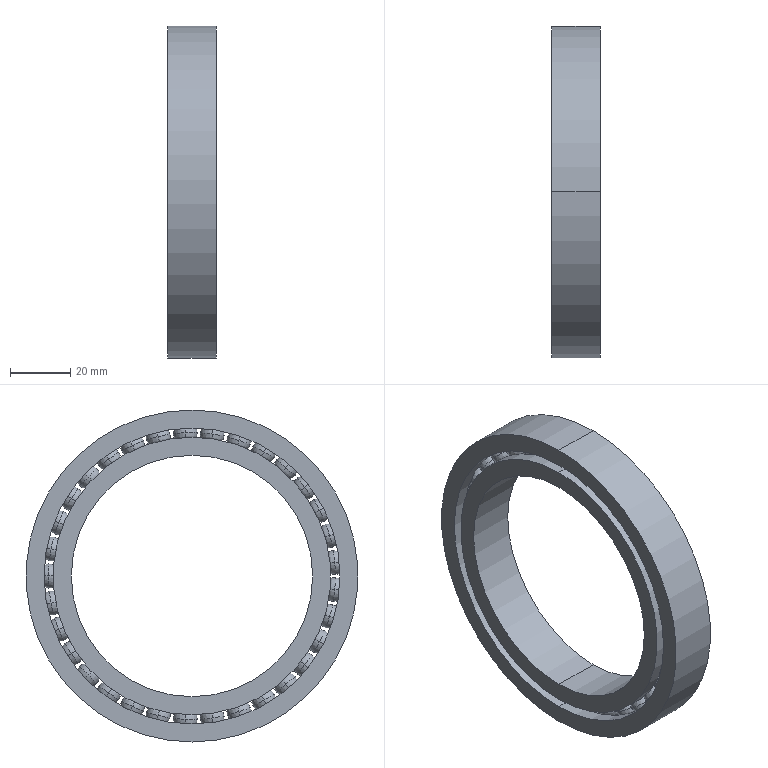Part | NX | features BREP 35 | 35 solids | 154 faces | box 16 x 110 x 110 mm | volume 58139 mm3 | sphere 132 | cylinder 12 | torus 6 | plane 4 | commonest cylinder face diameters 92 x4 98 x4 80 x2 110 x2